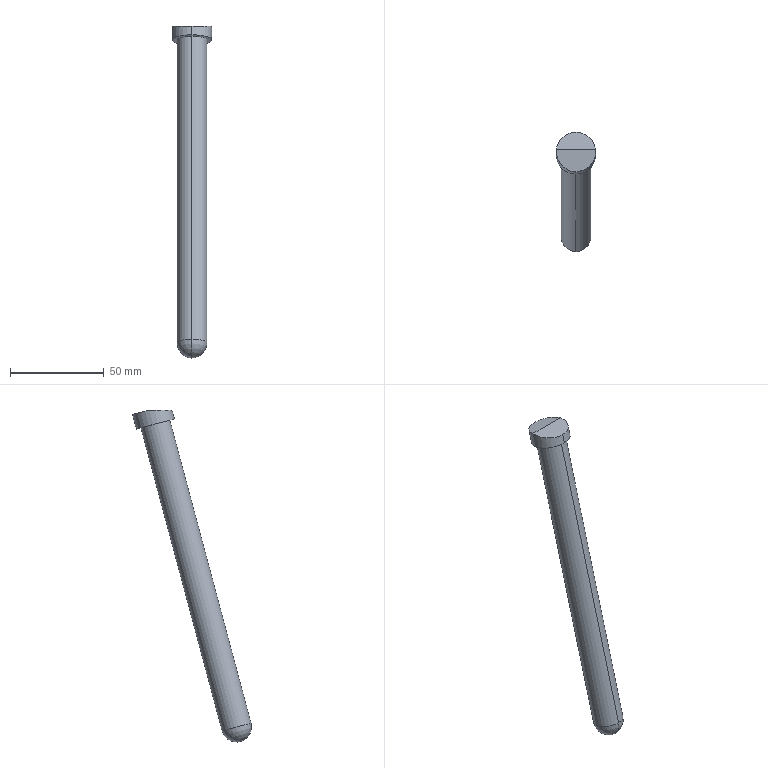Part | Creo | 1 solid | 9 faces | box 21.001 x 63.604 x 177.382 mm | volume 37290 mm3 | cylinder 4 | plane 3 | sphere 2 | commonest cylinder face diameters 16 x2 21 x2
STEP:
#1=CARTESIAN_POINT('',(0.,0.,0.));
#2=DIRECTION('',(0.,0.,1.));
#3=DIRECTION('',(1.,0.,0.));
#4=AXIS2_PLACEMENT_3D('',#1,#2,#3);
#5=CARTESIAN_POINT('',(10.393,-135.037,120.5));
#6=VERTEX_POINT('',#5);
#7=CARTESIAN_POINT('',(-0.05,-125.954,118.066));
#8=VERTEX_POINT('',#7);
#9=CARTESIAN_POINT('',(-0.05,-136.096,120.784));
#10=DIRECTION('',(0.,0.2588,0.9659));
#11=DIRECTION('',(0.9945,0.1008,-0.02702));
#12=AXIS2_PLACEMENT_3D('',#9,#10,#11);
#13=CIRCLE('',#12,10.5);
#14=EDGE_CURVE('',#6,#8,#13,.T.);
#15=ORIENTED_EDGE('',*,*,#14,.F.);
#16=CARTESIAN_POINT('',(-10.493,-135.037,120.5));
#17=VERTEX_POINT('',#16);
#18=CARTESIAN_POINT('',(10.393,-135.037,120.5));
#19=DIRECTION('',(-1.,-0.000000007,0.000000002));
#20=VECTOR('',#19,20.885);
#21=LINE('',#18,#20);
#22=EDGE_CURVE('',#6,#17,#21,.T.);
#23=ORIENTED_EDGE('',*,*,#22,.T.);
#24=CARTESIAN_POINT('',(-0.05,-136.096,120.784));
#25=DIRECTION('',(0.,0.2588,0.9659));
#26=DIRECTION('',(0.,0.9659,-0.2588));
#27=AXIS2_PLACEMENT_3D('',#24,#25,#26);
#28=CIRCLE('',#27,10.5);
#29=EDGE_CURVE('',#8,#17,#28,.T.);
#30=ORIENTED_EDGE('',*,*,#29,.F.);
#31=EDGE_LOOP('',(#15,#23,#30));
#32=FACE_OUTER_BOUND('',#31,.F.);
#33=CARTESIAN_POINT('',(-0.05,-146.238,123.501));
#34=DIRECTION('',(0.,0.2588,0.9659));
#35=DIRECTION('',(0.,-0.9659,0.2588));
#36=AXIS2_PLACEMENT_3D('',#33,#34,#35);
#37=PLANE('',#36);
#38=ADVANCED_FACE('',(#32),#37,.T.);
#39=CARTESIAN_POINT('',(-0.05,-128.024,110.339));
#40=VERTEX_POINT('',#39);
#41=CARTESIAN_POINT('',(-0.05,-148.309,115.774));
#42=VERTEX_POINT('',#41);
#43=CARTESIAN_POINT('',(-0.05,-138.167,113.056));
#44=DIRECTION('',(0.,-0.2588,-0.9659));
#45=DIRECTION('',(0.,0.9659,-0.2588));
#46=AXIS2_PLACEMENT_3D('',#43,#44,#45);
#47=CIRCLE('',#46,10.5);
#48=EDGE_CURVE('',#40,#42,#47,.T.);
#49=ORIENTED_EDGE('',*,*,#48,.T.);
#50=CARTESIAN_POINT('',(-0.05,-147.042,120.5));
#51=VERTEX_POINT('',#50);
#52=CARTESIAN_POINT('',(-0.05,-147.042,120.5));
#53=DIRECTION('',(-0.000000002,-0.2588,-0.9659));
#54=VECTOR('',#53,4.893);
#55=LINE('',#52,#54);
#56=EDGE_CURVE('',#51,#42,#55,.T.);
#57=ORIENTED_EDGE('',*,*,#56,.F.);
#58=CARTESIAN_POINT('',(-0.05,-147.042,120.5));
#59=CARTESIAN_POINT('',(0.5992,-147.042,120.5));
#60=CARTESIAN_POINT('',(1.871,-146.92,120.5));
#61=CARTESIAN_POINT('',(3.72,-146.382,120.5));
#62=CARTESIAN_POINT('',(5.449,-145.504,120.5));
#63=CARTESIAN_POINT('',(7.014,-144.299,120.5));
#64=CARTESIAN_POINT('',(8.34,-142.812,120.5));
#65=CARTESIAN_POINT('',(9.382,-141.092,120.5));
#66=CARTESIAN_POINT('',(10.109,-139.169,120.5));
#67=CARTESIAN_POINT('',(10.474,-137.118,120.5));
#68=CARTESIAN_POINT('',(10.464,-135.737,120.5));
#69=CARTESIAN_POINT('',(10.393,-135.037,120.5));
#70=B_SPLINE_CURVE_WITH_KNOTS('',3,(#58,#59,#60,#61,#62,#63,#64,#65,#66,#67,#68,#69),.UNSPECIFIED.,.F.,.F.,(4,1,1,1,1,1,1,1,1,4),(0.,0.1111,0.2222,0.3333,0.4444,0.5556,0.6667,0.7778,0.8889,1.),.UNSPECIFIED.);
#71=EDGE_CURVE('',#51,#6,#70,.T.);
#72=ORIENTED_EDGE('',*,*,#71,.T.);
#73=ORIENTED_EDGE('',*,*,#14,.T.);
#74=CARTESIAN_POINT('',(-0.05,-125.954,118.066));
#75=DIRECTION('',(0.,-0.2588,-0.9659));
#76=VECTOR('',#75,8.);
#77=LINE('',#74,#76);
#78=EDGE_CURVE('',#8,#40,#77,.T.);
#79=ORIENTED_EDGE('',*,*,#78,.T.);
#80=EDGE_LOOP('',(#49,#57,#72,#73,#79));
#81=FACE_OUTER_BOUND('',#80,.F.);
#82=CARTESIAN_POINT('',(-0.05,-189.686,-79.216));
#83=DIRECTION('',(0.,-0.2588,-0.9659));
#84=DIRECTION('',(0.,0.9659,-0.2588));
#85=AXIS2_PLACEMENT_3D('',#82,#83,#84);
#86=CYLINDRICAL_SURFACE('',#85,10.5);
#87=ADVANCED_FACE('',(#81),#86,.T.);
#88=CARTESIAN_POINT('',(-0.05,-138.167,113.056));
#89=DIRECTION('',(0.,-0.2588,-0.9659));
#90=DIRECTION('',(0.,-0.9659,0.2588));
#91=AXIS2_PLACEMENT_3D('',#88,#89,#90);
#92=CIRCLE('',#91,10.5);
#93=EDGE_CURVE('',#42,#40,#92,.T.);
#94=ORIENTED_EDGE('',*,*,#93,.F.);
#95=ORIENTED_EDGE('',*,*,#48,.F.);
#96=EDGE_LOOP('',(#94,#95));
#97=FACE_OUTER_BOUND('',#96,.F.);
#98=CARTESIAN_POINT('',(-0.05,-145.894,115.127));
#99=VERTEX_POINT('',#98);
#100=CARTESIAN_POINT('',(-0.05,-130.439,110.986));
#101=VERTEX_POINT('',#100);
#102=CARTESIAN_POINT('',(-0.05,-138.167,113.056));
#103=DIRECTION('',(0.,0.2588,0.9659));
#104=DIRECTION('',(0.,-0.9659,0.2588));
#105=AXIS2_PLACEMENT_3D('',#102,#103,#104);
#106=CIRCLE('',#105,8.);
#107=EDGE_CURVE('',#99,#101,#106,.T.);
#108=ORIENTED_EDGE('',*,*,#107,.F.);
#109=CARTESIAN_POINT('',(-0.05,-138.167,113.056));
#110=DIRECTION('',(0.,0.2588,0.9659));
#111=DIRECTION('',(0.,0.9659,-0.2588));
#112=AXIS2_PLACEMENT_3D('',#109,#110,#111);
#113=CIRCLE('',#112,8.);
#114=EDGE_CURVE('',#101,#99,#113,.T.);
#115=ORIENTED_EDGE('',*,*,#114,.F.);
#116=EDGE_LOOP('',(#108,#115));
#117=FACE_BOUND('',#116,.F.);
#118=CARTESIAN_POINT('',(-0.05,-145.894,115.127));
#119=DIRECTION('',(0.,-0.2588,-0.9659));
#120=DIRECTION('',(0.,0.9659,-0.2588));
#121=AXIS2_PLACEMENT_3D('',#118,#119,#120);
#122=PLANE('',#121);
#123=ADVANCED_FACE('',(#97,#117),#122,.T.);
#124=ORIENTED_EDGE('',*,*,#93,.T.);
#125=ORIENTED_EDGE('',*,*,#78,.F.);
#126=ORIENTED_EDGE('',*,*,#29,.T.);
#127=CARTESIAN_POINT('',(-10.493,-135.037,120.5));
#128=CARTESIAN_POINT('',(-10.571,-135.814,120.5));
#129=CARTESIAN_POINT('',(-10.567,-137.345,120.5));
#130=CARTESIAN_POINT('',(-10.091,-139.624,120.5));
#131=CARTESIAN_POINT('',(-9.163,-141.731,120.5));
#132=CARTESIAN_POINT('',(-7.854,-143.563,120.5));
#133=CARTESIAN_POINT('',(-6.184,-145.093,120.5));
#134=CARTESIAN_POINT('',(-4.272,-146.21,120.5));
#135=CARTESIAN_POINT('',(-2.198,-146.89,120.5));
#136=CARTESIAN_POINT('',(-0.7763,-147.042,120.5));
#137=CARTESIAN_POINT('',(-0.05,-147.042,120.5));
#138=B_SPLINE_CURVE_WITH_KNOTS('',3,(#127,#128,#129,#130,#131,#132,#133,#134,#135,#136,#137),.UNSPECIFIED.,.F.,.F.,(4,1,1,1,1,1,1,1,4),(0.,0.125,0.25,0.375,0.5,0.625,0.75,0.875,1.),.UNSPECIFIED.);
#139=EDGE_CURVE('',#17,#51,#138,.T.);
#140=ORIENTED_EDGE('',*,*,#139,.T.);
#141=ORIENTED_EDGE('',*,*,#56,.T.);
#142=EDGE_LOOP('',(#124,#125,#126,#140,#141));
#143=FACE_OUTER_BOUND('',#142,.F.);
#144=CARTESIAN_POINT('',(-0.05,-189.686,-79.216));
#145=DIRECTION('',(0.,-0.2588,-0.9659));
#146=DIRECTION('',(0.,0.9659,-0.2588));
#147=AXIS2_PLACEMENT_3D('',#144,#145,#146);
#148=CYLINDRICAL_SURFACE('',#147,10.5);
#149=ADVANCED_FACE('',(#143),#148,.T.);
#150=ORIENTED_EDGE('',*,*,#71,.F.);
#151=ORIENTED_EDGE('',*,*,#139,.F.);
#152=ORIENTED_EDGE('',*,*,#22,.F.);
#153=EDGE_LOOP('',(#150,#151,#152));
#154=FACE_OUTER_BOUND('',#153,.F.);
#155=CARTESIAN_POINT('',(200.,-250.,120.5));
#156=DIRECTION('',(0.,0.,1.));
#157=DIRECTION('',(-1.,0.,0.));
#158=AXIS2_PLACEMENT_3D('',#155,#156,#157);
#159=PLANE('',#158);
#160=ADVANCED_FACE('',(#154),#159,.T.);
#161=ORIENTED_EDGE('',*,*,#107,.T.);
#162=CARTESIAN_POINT('',(-0.05,-173.831,-50.953));
#163=VERTEX_POINT('',#162);
#164=CARTESIAN_POINT('',(-0.05,-130.439,110.986));
#165=DIRECTION('',(0.,-0.2588,-0.9659));
#166=VECTOR('',#165,167.651);
#167=LINE('',#164,#166);
#168=EDGE_CURVE('',#101,#163,#167,.T.);
#169=ORIENTED_EDGE('',*,*,#168,.T.);
#170=CARTESIAN_POINT('',(-0.05,-189.285,-46.812));
#171=VERTEX_POINT('',#170);
#172=CARTESIAN_POINT('',(-0.05,-181.558,-48.882));
#173=DIRECTION('',(0.,-0.2588,-0.9659));
#174=DIRECTION('',(0.,0.9659,-0.2588));
#175=AXIS2_PLACEMENT_3D('',#172,#173,#174);
#176=CIRCLE('',#175,8.);
#177=EDGE_CURVE('',#163,#171,#176,.T.);
#178=ORIENTED_EDGE('',*,*,#177,.T.);
#179=CARTESIAN_POINT('',(-0.05,-145.894,115.127));
#180=DIRECTION('',(0.,-0.2588,-0.9659));
#181=VECTOR('',#180,167.651);
#182=LINE('',#179,#181);
#183=EDGE_CURVE('',#99,#171,#182,.T.);
#184=ORIENTED_EDGE('',*,*,#183,.F.);
#185=EDGE_LOOP('',(#161,#169,#178,#184));
#186=FACE_OUTER_BOUND('',#185,.F.);
#187=CARTESIAN_POINT('',(-0.05,-183.733,-57.));
#188=DIRECTION('',(0.,-0.2588,-0.9659));
#189=DIRECTION('',(0.,0.9659,-0.2588));
#190=AXIS2_PLACEMENT_3D('',#187,#188,#189);
#191=CYLINDRICAL_SURFACE('',#190,8.);
#192=ADVANCED_FACE('',(#186),#191,.T.);
#193=ORIENTED_EDGE('',*,*,#114,.T.);
#194=ORIENTED_EDGE('',*,*,#183,.T.);
#195=CARTESIAN_POINT('',(-0.05,-181.558,-48.882));
#196=DIRECTION('',(0.,-0.2588,-0.9659));
#197=DIRECTION('',(0.,-0.9659,0.2588));
#198=AXIS2_PLACEMENT_3D('',#195,#196,#197);
#199=CIRCLE('',#198,8.);
#200=EDGE_CURVE('',#171,#163,#199,.T.);
#201=ORIENTED_EDGE('',*,*,#200,.T.);
#202=ORIENTED_EDGE('',*,*,#168,.F.);
#203=EDGE_LOOP('',(#193,#194,#201,#202));
#204=FACE_OUTER_BOUND('',#203,.F.);
#205=CARTESIAN_POINT('',(-0.05,-183.733,-57.));
#206=DIRECTION('',(0.,-0.2588,-0.9659));
#207=DIRECTION('',(0.,0.9659,-0.2588));
#208=AXIS2_PLACEMENT_3D('',#205,#206,#207);
#209=CYLINDRICAL_SURFACE('',#208,8.);
#210=ADVANCED_FACE('',(#204),#209,.T.);
#211=ORIENTED_EDGE('',*,*,#200,.F.);
#212=CARTESIAN_POINT('',(-0.05,-183.628,-56.61));
#213=VERTEX_POINT('',#212);
#214=CARTESIAN_POINT('',(-0.05,-181.558,-48.882));
#215=DIRECTION('',(1.,0.,0.));
#216=DIRECTION('',(0.,-0.9659,0.2588));
#217=AXIS2_PLACEMENT_3D('',#214,#215,#216);
#218=CIRCLE('',#217,8.);
#219=EDGE_CURVE('',#171,#213,#218,.T.);
#220=ORIENTED_EDGE('',*,*,#219,.T.);
#221=CARTESIAN_POINT('',(-0.05,-181.558,-48.882));
#222=DIRECTION('',(-1.,0.,0.));
#223=DIRECTION('',(0.,0.9659,-0.2588));
#224=AXIS2_PLACEMENT_3D('',#221,#222,#223);
#225=CIRCLE('',#224,8.);
#226=EDGE_CURVE('',#163,#213,#225,.T.);
#227=ORIENTED_EDGE('',*,*,#226,.F.);
#228=EDGE_LOOP('',(#211,#220,#227));
#229=FACE_OUTER_BOUND('',#228,.F.);
#230=CARTESIAN_POINT('',(-0.05,-181.558,-48.882));
#231=DIRECTION('',(0.,-0.2588,-0.9659));
#232=DIRECTION('',(0.,0.9659,-0.2588));
#233=AXIS2_PLACEMENT_3D('',#230,#231,#232);
#234=SPHERICAL_SURFACE('',#233,8.);
#235=ADVANCED_FACE('',(#229),#234,.T.);
#236=ORIENTED_EDGE('',*,*,#177,.F.);
#237=ORIENTED_EDGE('',*,*,#226,.T.);
#238=ORIENTED_EDGE('',*,*,#219,.F.);
#239=EDGE_LOOP('',(#236,#237,#238));
#240=FACE_OUTER_BOUND('',#239,.F.);
#241=CARTESIAN_POINT('',(-0.05,-181.558,-48.882));
#242=DIRECTION('',(0.,-0.2588,-0.9659));
#243=DIRECTION('',(0.,0.9659,-0.2588));
#244=AXIS2_PLACEMENT_3D('',#241,#242,#243);
#245=SPHERICAL_SURFACE('',#244,8.);
#246=ADVANCED_FACE('',(#240),#245,.T.);
#247=CLOSED_SHELL('',(#38,#87,#123,#149,#160,#192,#210,#235,#246));
#248=MANIFOLD_SOLID_BREP('',#247);
#249=(LENGTH_UNIT()NAMED_UNIT(*)SI_UNIT(.MILLI.,.METRE.));
#250=UNCERTAINTY_MEASURE_WITH_UNIT(LENGTH_MEASURE(0.01924),#249,'','');
#251=(NAMED_UNIT(*)PLANE_ANGLE_UNIT()SI_UNIT($,.RADIAN.));
#252=PLANE_ANGLE_MEASURE_WITH_UNIT(PLANE_ANGLE_MEASURE(0.01745),#251);
#253=(CONVERSION_BASED_UNIT('DEGREE',#252)NAMED_UNIT(*)PLANE_ANGLE_UNIT());
#254=(NAMED_UNIT(*)SI_UNIT($,.STERADIAN.)SOLID_ANGLE_UNIT());
#255=(GEOMETRIC_REPRESENTATION_CONTEXT(3)GLOBAL_UNCERTAINTY_ASSIGNED_CONTEXT((#250))GLOBAL_UNIT_ASSIGNED_CONTEXT((#249,#253,#254))REPRESENTATION_CONTEXT('',''));
#256=ADVANCED_BREP_SHAPE_REPRESENTATION('',(#4,#248),#255);